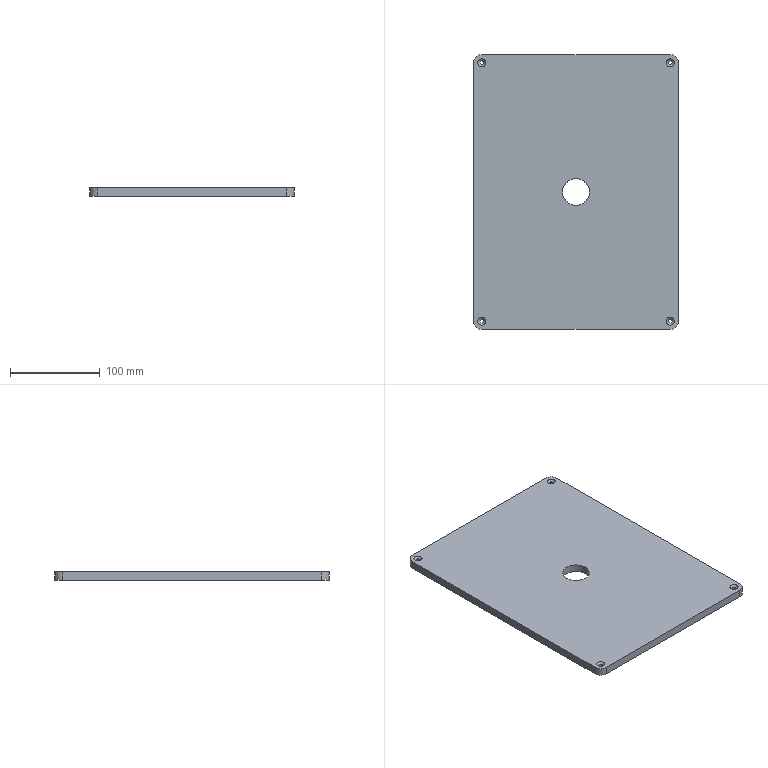Part | STEP file | Substructure | 1 solid | 19 faces | box 228 x 306 x 9 mm | volume 620161 mm3 | cylinder 9 | plane 6 | cone 4 | commonest cylinder face diameters 4.5 x4 18 x4 30 x1
STEP:
#1=CARTESIAN_POINT('',(0.,0.,0.));
#2=DIRECTION('',(0.,0.,1.));
#3=DIRECTION('',(1.,0.,0.));
#4=AXIS2_PLACEMENT_3D('',#1,#2,#3);
#5=CARTESIAN_POINT('',(-105.,-153.,0.));
#6=VERTEX_POINT('',#5);
#7=CARTESIAN_POINT('',(-105.,-153.,-9.));
#8=VERTEX_POINT('',#7);
#9=CARTESIAN_POINT('',(-105.,-153.,0.));
#10=DIRECTION('',(0.,0.,-1.));
#11=VECTOR('',#10,1.);
#12=LINE('',#9,#11);
#13=CARTESIAN_POINT('',(-105.,-153.,0.));
#14=DIRECTION('',(0.,-1.,0.));
#15=DIRECTION('',(1.,0.,0.));
#16=AXIS2_PLACEMENT_3D('',#13,#14,#15);
#17=PLANE('',#16);
#18=CARTESIAN_POINT('',(0.,0.));
#19=DIRECTION('',(0.,-1.));
#20=VECTOR('',#19,1.);
#21=LINE('',#18,#20);
#22=(GEOMETRIC_REPRESENTATION_CONTEXT(2)PARAMETRIC_REPRESENTATION_CONTEXT()REPRESENTATION_CONTEXT('',''));
#23=DEFINITIONAL_REPRESENTATION('',(#21),#22);
#24=PCURVE('',#17,#23);
#25=CARTESIAN_POINT('',(-105.,-144.,0.));
#26=DIRECTION('',(0.,0.,1.));
#27=DIRECTION('',(1.,0.,0.));
#28=AXIS2_PLACEMENT_3D('',#25,#26,#27);
#29=CYLINDRICAL_SURFACE('',#28,9.);
#30=CARTESIAN_POINT('',(4.712,0.));
#31=DIRECTION('',(0.,-1.));
#32=VECTOR('',#31,1.);
#33=LINE('',#30,#32);
#34=(GEOMETRIC_REPRESENTATION_CONTEXT(2)PARAMETRIC_REPRESENTATION_CONTEXT()REPRESENTATION_CONTEXT('',''));
#35=DEFINITIONAL_REPRESENTATION('',(#33),#34);
#36=PCURVE('',#29,#35);
#37=SURFACE_CURVE('',#12,(#24,#36),.PCURVE_S1.);
#38=EDGE_CURVE('',#6,#8,#37,.T.);
#39=ORIENTED_EDGE('',*,*,#38,.T.);
#40=CARTESIAN_POINT('',(105.,-153.,-9.));
#41=VERTEX_POINT('',#40);
#42=CARTESIAN_POINT('',(-105.,-153.,-9.));
#43=DIRECTION('',(1.,0.,0.));
#44=VECTOR('',#43,1.);
#45=LINE('',#42,#44);
#46=CARTESIAN_POINT('',(0.,-9.));
#47=DIRECTION('',(1.,0.));
#48=VECTOR('',#47,1.);
#49=LINE('',#46,#48);
#50=(GEOMETRIC_REPRESENTATION_CONTEXT(2)PARAMETRIC_REPRESENTATION_CONTEXT()REPRESENTATION_CONTEXT('',''));
#51=DEFINITIONAL_REPRESENTATION('',(#49),#50);
#52=PCURVE('',#17,#51);
#53=CARTESIAN_POINT('',(0.,0.,-9.));
#54=DIRECTION('',(0.,0.,1.));
#55=DIRECTION('',(1.,0.,0.));
#56=AXIS2_PLACEMENT_3D('',#53,#54,#55);
#57=PLANE('',#56);
#58=CARTESIAN_POINT('',(-105.,-153.));
#59=DIRECTION('',(1.,0.));
#60=VECTOR('',#59,1.);
#61=LINE('',#58,#60);
#62=(GEOMETRIC_REPRESENTATION_CONTEXT(2)PARAMETRIC_REPRESENTATION_CONTEXT()REPRESENTATION_CONTEXT('',''));
#63=DEFINITIONAL_REPRESENTATION('',(#61),#62);
#64=PCURVE('',#57,#63);
#65=SURFACE_CURVE('',#45,(#52,#64),.PCURVE_S1.);
#66=EDGE_CURVE('',#8,#41,#65,.T.);
#67=ORIENTED_EDGE('',*,*,#66,.T.);
#68=CARTESIAN_POINT('',(105.,-153.,0.));
#69=VERTEX_POINT('',#68);
#70=CARTESIAN_POINT('',(105.,-153.,0.));
#71=DIRECTION('',(0.,0.,-1.));
#72=VECTOR('',#71,1.);
#73=LINE('',#70,#72);
#74=CARTESIAN_POINT('',(210.,0.));
#75=DIRECTION('',(0.,-1.));
#76=VECTOR('',#75,1.);
#77=LINE('',#74,#76);
#78=(GEOMETRIC_REPRESENTATION_CONTEXT(2)PARAMETRIC_REPRESENTATION_CONTEXT()REPRESENTATION_CONTEXT('',''));
#79=DEFINITIONAL_REPRESENTATION('',(#77),#78);
#80=PCURVE('',#17,#79);
#81=CARTESIAN_POINT('',(105.,-144.,0.));
#82=DIRECTION('',(0.,0.,1.));
#83=DIRECTION('',(1.,0.,0.));
#84=AXIS2_PLACEMENT_3D('',#81,#82,#83);
#85=CYLINDRICAL_SURFACE('',#84,9.);
#86=CARTESIAN_POINT('',(4.712,0.));
#87=DIRECTION('',(0.,-1.));
#88=VECTOR('',#87,1.);
#89=LINE('',#86,#88);
#90=(GEOMETRIC_REPRESENTATION_CONTEXT(2)PARAMETRIC_REPRESENTATION_CONTEXT()REPRESENTATION_CONTEXT('',''));
#91=DEFINITIONAL_REPRESENTATION('',(#89),#90);
#92=PCURVE('',#85,#91);
#93=SURFACE_CURVE('',#73,(#80,#92),.PCURVE_S1.);
#94=EDGE_CURVE('',#69,#41,#93,.T.);
#95=ORIENTED_EDGE('',*,*,#94,.F.);
#96=CARTESIAN_POINT('',(-105.,-153.,0.));
#97=DIRECTION('',(1.,0.,0.));
#98=VECTOR('',#97,1.);
#99=LINE('',#96,#98);
#100=CARTESIAN_POINT('',(0.,0.));
#101=DIRECTION('',(1.,0.));
#102=VECTOR('',#101,1.);
#103=LINE('',#100,#102);
#104=(GEOMETRIC_REPRESENTATION_CONTEXT(2)PARAMETRIC_REPRESENTATION_CONTEXT()REPRESENTATION_CONTEXT('',''));
#105=DEFINITIONAL_REPRESENTATION('',(#103),#104);
#106=PCURVE('',#17,#105);
#107=CARTESIAN_POINT('',(0.,0.,0.));
#108=DIRECTION('',(0.,0.,1.));
#109=DIRECTION('',(1.,0.,0.));
#110=AXIS2_PLACEMENT_3D('',#107,#108,#109);
#111=PLANE('',#110);
#112=CARTESIAN_POINT('',(-105.,-153.));
#113=DIRECTION('',(1.,0.));
#114=VECTOR('',#113,1.);
#115=LINE('',#112,#114);
#116=(GEOMETRIC_REPRESENTATION_CONTEXT(2)PARAMETRIC_REPRESENTATION_CONTEXT()REPRESENTATION_CONTEXT('',''));
#117=DEFINITIONAL_REPRESENTATION('',(#115),#116);
#118=PCURVE('',#111,#117);
#119=SURFACE_CURVE('',#99,(#106,#118),.PCURVE_S1.);
#120=EDGE_CURVE('',#6,#69,#119,.T.);
#121=ORIENTED_EDGE('',*,*,#120,.F.);
#122=EDGE_LOOP('',(#39,#67,#95,#121));
#123=FACE_BOUND('',#122,.T.);
#124=ADVANCED_FACE('',(#123),#17,.T.);
#125=CARTESIAN_POINT('',(-114.,-144.,0.));
#126=VERTEX_POINT('',#125);
#127=CARTESIAN_POINT('',(-114.,-144.,-9.));
#128=VERTEX_POINT('',#127);
#129=CARTESIAN_POINT('',(-114.,-144.,0.));
#130=DIRECTION('',(0.,0.,-1.));
#131=VECTOR('',#130,1.);
#132=LINE('',#129,#131);
#133=CARTESIAN_POINT('',(3.142,0.));
#134=DIRECTION('',(0.,-1.));
#135=VECTOR('',#134,1.);
#136=LINE('',#133,#135);
#137=(GEOMETRIC_REPRESENTATION_CONTEXT(2)PARAMETRIC_REPRESENTATION_CONTEXT()REPRESENTATION_CONTEXT('',''));
#138=DEFINITIONAL_REPRESENTATION('',(#136),#137);
#139=PCURVE('',#29,#138);
#140=CARTESIAN_POINT('',(-114.,144.,0.));
#141=DIRECTION('',(-1.,0.,0.));
#142=DIRECTION('',(0.,-1.,0.));
#143=AXIS2_PLACEMENT_3D('',#140,#141,#142);
#144=PLANE('',#143);
#145=CARTESIAN_POINT('',(288.,0.));
#146=DIRECTION('',(0.,-1.));
#147=VECTOR('',#146,1.);
#148=LINE('',#145,#147);
#149=(GEOMETRIC_REPRESENTATION_CONTEXT(2)PARAMETRIC_REPRESENTATION_CONTEXT()REPRESENTATION_CONTEXT('',''));
#150=DEFINITIONAL_REPRESENTATION('',(#148),#149);
#151=PCURVE('',#144,#150);
#152=SURFACE_CURVE('',#132,(#139,#151),.PCURVE_S1.);
#153=EDGE_CURVE('',#126,#128,#152,.T.);
#154=ORIENTED_EDGE('',*,*,#153,.T.);
#155=CARTESIAN_POINT('',(-105.,-144.,-9.));
#156=DIRECTION('',(0.,0.,1.));
#157=DIRECTION('',(1.,0.,0.));
#158=AXIS2_PLACEMENT_3D('',#155,#156,#157);
#159=CIRCLE('',#158,9.);
#160=CARTESIAN_POINT('',(0.,-9.));
#161=DIRECTION('',(1.,0.));
#162=VECTOR('',#161,1.);
#163=LINE('',#160,#162);
#164=(GEOMETRIC_REPRESENTATION_CONTEXT(2)PARAMETRIC_REPRESENTATION_CONTEXT()REPRESENTATION_CONTEXT('',''));
#165=DEFINITIONAL_REPRESENTATION('',(#163),#164);
#166=PCURVE('',#29,#165);
#167=CARTESIAN_POINT('',(-105.,-144.));
#168=DIRECTION('',(1.,0.));
#169=AXIS2_PLACEMENT_2D('',#167,#168);
#170=CIRCLE('',#169,9.);
#171=(GEOMETRIC_REPRESENTATION_CONTEXT(2)PARAMETRIC_REPRESENTATION_CONTEXT()REPRESENTATION_CONTEXT('',''));
#172=DEFINITIONAL_REPRESENTATION('',(#170),#171);
#173=PCURVE('',#57,#172);
#174=SURFACE_CURVE('',#159,(#166,#173),.PCURVE_S1.);
#175=EDGE_CURVE('',#128,#8,#174,.T.);
#176=ORIENTED_EDGE('',*,*,#175,.T.);
#177=ORIENTED_EDGE('',*,*,#38,.F.);
#178=CARTESIAN_POINT('',(-105.,-144.,0.));
#179=DIRECTION('',(0.,0.,1.));
#180=DIRECTION('',(1.,0.,0.));
#181=AXIS2_PLACEMENT_3D('',#178,#179,#180);
#182=CIRCLE('',#181,9.);
#183=CARTESIAN_POINT('',(0.,0.));
#184=DIRECTION('',(1.,0.));
#185=VECTOR('',#184,1.);
#186=LINE('',#183,#185);
#187=(GEOMETRIC_REPRESENTATION_CONTEXT(2)PARAMETRIC_REPRESENTATION_CONTEXT()REPRESENTATION_CONTEXT('',''));
#188=DEFINITIONAL_REPRESENTATION('',(#186),#187);
#189=PCURVE('',#29,#188);
#190=CARTESIAN_POINT('',(-105.,-144.));
#191=DIRECTION('',(1.,0.));
#192=AXIS2_PLACEMENT_2D('',#190,#191);
#193=CIRCLE('',#192,9.);
#194=(GEOMETRIC_REPRESENTATION_CONTEXT(2)PARAMETRIC_REPRESENTATION_CONTEXT()REPRESENTATION_CONTEXT('',''));
#195=DEFINITIONAL_REPRESENTATION('',(#193),#194);
#196=PCURVE('',#111,#195);
#197=SURFACE_CURVE('',#182,(#189,#196),.PCURVE_S1.);
#198=EDGE_CURVE('',#126,#6,#197,.T.);
#199=ORIENTED_EDGE('',*,*,#198,.F.);
#200=EDGE_LOOP('',(#154,#176,#177,#199));
#201=FACE_BOUND('',#200,.T.);
#202=ADVANCED_FACE('',(#201),#29,.T.);
#203=ORIENTED_EDGE('',*,*,#94,.T.);
#204=CARTESIAN_POINT('',(114.,-144.,-9.));
#205=VERTEX_POINT('',#204);
#206=CARTESIAN_POINT('',(105.,-144.,-9.));
#207=DIRECTION('',(0.,0.,1.));
#208=DIRECTION('',(1.,0.,0.));
#209=AXIS2_PLACEMENT_3D('',#206,#207,#208);
#210=CIRCLE('',#209,9.);
#211=CARTESIAN_POINT('',(0.,-9.));
#212=DIRECTION('',(1.,0.));
#213=VECTOR('',#212,1.);
#214=LINE('',#211,#213);
#215=(GEOMETRIC_REPRESENTATION_CONTEXT(2)PARAMETRIC_REPRESENTATION_CONTEXT()REPRESENTATION_CONTEXT('',''));
#216=DEFINITIONAL_REPRESENTATION('',(#214),#215);
#217=PCURVE('',#85,#216);
#218=CARTESIAN_POINT('',(105.,-144.));
#219=DIRECTION('',(1.,0.));
#220=AXIS2_PLACEMENT_2D('',#218,#219);
#221=CIRCLE('',#220,9.);
#222=(GEOMETRIC_REPRESENTATION_CONTEXT(2)PARAMETRIC_REPRESENTATION_CONTEXT()REPRESENTATION_CONTEXT('',''));
#223=DEFINITIONAL_REPRESENTATION('',(#221),#222);
#224=PCURVE('',#57,#223);
#225=SURFACE_CURVE('',#210,(#217,#224),.PCURVE_S1.);
#226=EDGE_CURVE('',#41,#205,#225,.T.);
#227=ORIENTED_EDGE('',*,*,#226,.T.);
#228=CARTESIAN_POINT('',(114.,-144.,0.));
#229=VERTEX_POINT('',#228);
#230=CARTESIAN_POINT('',(114.,-144.,0.));
#231=DIRECTION('',(0.,0.,-1.));
#232=VECTOR('',#231,1.);
#233=LINE('',#230,#232);
#234=CARTESIAN_POINT('',(6.283,0.));
#235=DIRECTION('',(0.,-1.));
#236=VECTOR('',#235,1.);
#237=LINE('',#234,#236);
#238=(GEOMETRIC_REPRESENTATION_CONTEXT(2)PARAMETRIC_REPRESENTATION_CONTEXT()REPRESENTATION_CONTEXT('',''));
#239=DEFINITIONAL_REPRESENTATION('',(#237),#238);
#240=PCURVE('',#85,#239);
#241=CARTESIAN_POINT('',(114.,-144.,0.));
#242=DIRECTION('',(1.,0.,0.));
#243=DIRECTION('',(0.,1.,0.));
#244=AXIS2_PLACEMENT_3D('',#241,#242,#243);
#245=PLANE('',#244);
#246=CARTESIAN_POINT('',(0.,0.));
#247=DIRECTION('',(0.,-1.));
#248=VECTOR('',#247,1.);
#249=LINE('',#246,#248);
#250=(GEOMETRIC_REPRESENTATION_CONTEXT(2)PARAMETRIC_REPRESENTATION_CONTEXT()REPRESENTATION_CONTEXT('',''));
#251=DEFINITIONAL_REPRESENTATION('',(#249),#250);
#252=PCURVE('',#245,#251);
#253=SURFACE_CURVE('',#233,(#240,#252),.PCURVE_S1.);
#254=EDGE_CURVE('',#229,#205,#253,.T.);
#255=ORIENTED_EDGE('',*,*,#254,.F.);
#256=CARTESIAN_POINT('',(105.,-144.,0.));
#257=DIRECTION('',(0.,0.,1.));
#258=DIRECTION('',(1.,0.,0.));
#259=AXIS2_PLACEMENT_3D('',#256,#257,#258);
#260=CIRCLE('',#259,9.);
#261=CARTESIAN_POINT('',(0.,0.));
#262=DIRECTION('',(1.,0.));
#263=VECTOR('',#262,1.);
#264=LINE('',#261,#263);
#265=(GEOMETRIC_REPRESENTATION_CONTEXT(2)PARAMETRIC_REPRESENTATION_CONTEXT()REPRESENTATION_CONTEXT('',''));
#266=DEFINITIONAL_REPRESENTATION('',(#264),#265);
#267=PCURVE('',#85,#266);
#268=CARTESIAN_POINT('',(105.,-144.));
#269=DIRECTION('',(1.,0.));
#270=AXIS2_PLACEMENT_2D('',#268,#269);
#271=CIRCLE('',#270,9.);
#272=(GEOMETRIC_REPRESENTATION_CONTEXT(2)PARAMETRIC_REPRESENTATION_CONTEXT()REPRESENTATION_CONTEXT('',''));
#273=DEFINITIONAL_REPRESENTATION('',(#271),#272);
#274=PCURVE('',#111,#273);
#275=SURFACE_CURVE('',#260,(#267,#274),.PCURVE_S1.);
#276=EDGE_CURVE('',#69,#229,#275,.T.);
#277=ORIENTED_EDGE('',*,*,#276,.F.);
#278=EDGE_LOOP('',(#203,#227,#255,#277));
#279=FACE_BOUND('',#278,.T.);
#280=ADVANCED_FACE('',(#279),#85,.T.);
#281=ORIENTED_EDGE('',*,*,#120,.T.);
#282=ORIENTED_EDGE('',*,*,#276,.T.);
#283=CARTESIAN_POINT('',(114.,144.,0.));
#284=VERTEX_POINT('',#283);
#285=CARTESIAN_POINT('',(114.,-144.,0.));
#286=DIRECTION('',(0.,1.,0.));
#287=VECTOR('',#286,1.);
#288=LINE('',#285,#287);
#289=CARTESIAN_POINT('',(114.,-144.));
#290=DIRECTION('',(0.,1.));
#291=VECTOR('',#290,1.);
#292=LINE('',#289,#291);
#293=(GEOMETRIC_REPRESENTATION_CONTEXT(2)PARAMETRIC_REPRESENTATION_CONTEXT()REPRESENTATION_CONTEXT('',''));
#294=DEFINITIONAL_REPRESENTATION('',(#292),#293);
#295=PCURVE('',#111,#294);
#296=CARTESIAN_POINT('',(0.,0.));
#297=DIRECTION('',(1.,0.));
#298=VECTOR('',#297,1.);
#299=LINE('',#296,#298);
#300=(GEOMETRIC_REPRESENTATION_CONTEXT(2)PARAMETRIC_REPRESENTATION_CONTEXT()REPRESENTATION_CONTEXT('',''));
#301=DEFINITIONAL_REPRESENTATION('',(#299),#300);
#302=PCURVE('',#245,#301);
#303=SURFACE_CURVE('',#288,(#295,#302),.PCURVE_S1.);
#304=EDGE_CURVE('',#229,#284,#303,.T.);
#305=ORIENTED_EDGE('',*,*,#304,.T.);
#306=CARTESIAN_POINT('',(105.,153.,0.));
#307=VERTEX_POINT('',#306);
#308=CARTESIAN_POINT('',(105.,144.,0.));
#309=DIRECTION('',(0.,0.,1.));
#310=DIRECTION('',(1.,0.,0.));
#311=AXIS2_PLACEMENT_3D('',#308,#309,#310);
#312=CIRCLE('',#311,9.);
#313=CARTESIAN_POINT('',(105.,144.));
#314=DIRECTION('',(1.,0.));
#315=AXIS2_PLACEMENT_2D('',#313,#314);
#316=CIRCLE('',#315,9.);
#317=(GEOMETRIC_REPRESENTATION_CONTEXT(2)PARAMETRIC_REPRESENTATION_CONTEXT()REPRESENTATION_CONTEXT('',''));
#318=DEFINITIONAL_REPRESENTATION('',(#316),#317);
#319=PCURVE('',#111,#318);
#320=CARTESIAN_POINT('',(105.,144.,0.));
#321=DIRECTION('',(0.,0.,1.));
#322=DIRECTION('',(1.,0.,0.));
#323=AXIS2_PLACEMENT_3D('',#320,#321,#322);
#324=CYLINDRICAL_SURFACE('',#323,9.);
#325=CARTESIAN_POINT('',(0.,0.));
#326=DIRECTION('',(1.,0.));
#327=VECTOR('',#326,1.);
#328=LINE('',#325,#327);
#329=(GEOMETRIC_REPRESENTATION_CONTEXT(2)PARAMETRIC_REPRESENTATION_CONTEXT()REPRESENTATION_CONTEXT('',''));
#330=DEFINITIONAL_REPRESENTATION('',(#328),#329);
#331=PCURVE('',#324,#330);
#332=SURFACE_CURVE('',#312,(#319,#331),.PCURVE_S1.);
#333=EDGE_CURVE('',#284,#307,#332,.T.);
#334=ORIENTED_EDGE('',*,*,#333,.T.);
#335=CARTESIAN_POINT('',(-105.,153.,0.));
#336=VERTEX_POINT('',#335);
#337=CARTESIAN_POINT('',(105.,153.,0.));
#338=DIRECTION('',(-1.,0.,0.));
#339=VECTOR('',#338,1.);
#340=LINE('',#337,#339);
#341=CARTESIAN_POINT('',(105.,153.));
#342=DIRECTION('',(-1.,0.));
#343=VECTOR('',#342,1.);
#344=LINE('',#341,#343);
#345=(GEOMETRIC_REPRESENTATION_CONTEXT(2)PARAMETRIC_REPRESENTATION_CONTEXT()REPRESENTATION_CONTEXT('',''));
#346=DEFINITIONAL_REPRESENTATION('',(#344),#345);
#347=PCURVE('',#111,#346);
#348=CARTESIAN_POINT('',(105.,153.,0.));
#349=DIRECTION('',(0.,1.,0.));
#350=DIRECTION('',(-1.,0.,0.));
#351=AXIS2_PLACEMENT_3D('',#348,#349,#350);
#352=PLANE('',#351);
#353=CARTESIAN_POINT('',(0.,0.));
#354=DIRECTION('',(1.,0.));
#355=VECTOR('',#354,1.);
#356=LINE('',#353,#355);
#357=(GEOMETRIC_REPRESENTATION_CONTEXT(2)PARAMETRIC_REPRESENTATION_CONTEXT()REPRESENTATION_CONTEXT('',''));
#358=DEFINITIONAL_REPRESENTATION('',(#356),#357);
#359=PCURVE('',#352,#358);
#360=SURFACE_CURVE('',#340,(#347,#359),.PCURVE_S1.);
#361=EDGE_CURVE('',#307,#336,#360,.T.);
#362=ORIENTED_EDGE('',*,*,#361,.T.);
#363=CARTESIAN_POINT('',(-114.,144.,0.));
#364=VERTEX_POINT('',#363);
#365=CARTESIAN_POINT('',(-105.,144.,0.));
#366=DIRECTION('',(0.,0.,1.));
#367=DIRECTION('',(1.,0.,0.));
#368=AXIS2_PLACEMENT_3D('',#365,#366,#367);
#369=CIRCLE('',#368,9.);
#370=CARTESIAN_POINT('',(-105.,144.));
#371=DIRECTION('',(1.,0.));
#372=AXIS2_PLACEMENT_2D('',#370,#371);
#373=CIRCLE('',#372,9.);
#374=(GEOMETRIC_REPRESENTATION_CONTEXT(2)PARAMETRIC_REPRESENTATION_CONTEXT()REPRESENTATION_CONTEXT('',''));
#375=DEFINITIONAL_REPRESENTATION('',(#373),#374);
#376=PCURVE('',#111,#375);
#377=CARTESIAN_POINT('',(-105.,144.,0.));
#378=DIRECTION('',(0.,0.,1.));
#379=DIRECTION('',(1.,0.,0.));
#380=AXIS2_PLACEMENT_3D('',#377,#378,#379);
#381=CYLINDRICAL_SURFACE('',#380,9.);
#382=CARTESIAN_POINT('',(0.,0.));
#383=DIRECTION('',(1.,0.));
#384=VECTOR('',#383,1.);
#385=LINE('',#382,#384);
#386=(GEOMETRIC_REPRESENTATION_CONTEXT(2)PARAMETRIC_REPRESENTATION_CONTEXT()REPRESENTATION_CONTEXT('',''));
#387=DEFINITIONAL_REPRESENTATION('',(#385),#386);
#388=PCURVE('',#381,#387);
#389=SURFACE_CURVE('',#369,(#376,#388),.PCURVE_S1.);
#390=EDGE_CURVE('',#336,#364,#389,.T.);
#391=ORIENTED_EDGE('',*,*,#390,.T.);
#392=CARTESIAN_POINT('',(-114.,144.,0.));
#393=DIRECTION('',(0.,-1.,0.));
#394=VECTOR('',#393,1.);
#395=LINE('',#392,#394);
#396=CARTESIAN_POINT('',(-114.,144.));
#397=DIRECTION('',(0.,-1.));
#398=VECTOR('',#397,1.);
#399=LINE('',#396,#398);
#400=(GEOMETRIC_REPRESENTATION_CONTEXT(2)PARAMETRIC_REPRESENTATION_CONTEXT()REPRESENTATION_CONTEXT('',''));
#401=DEFINITIONAL_REPRESENTATION('',(#399),#400);
#402=PCURVE('',#111,#401);
#403=CARTESIAN_POINT('',(0.,0.));
#404=DIRECTION('',(1.,0.));
#405=VECTOR('',#404,1.);
#406=LINE('',#403,#405);
#407=(GEOMETRIC_REPRESENTATION_CONTEXT(2)PARAMETRIC_REPRESENTATION_CONTEXT()REPRESENTATION_CONTEXT('',''));
#408=DEFINITIONAL_REPRESENTATION('',(#406),#407);
#409=PCURVE('',#144,#408);
#410=SURFACE_CURVE('',#395,(#402,#409),.PCURVE_S1.);
#411=EDGE_CURVE('',#364,#126,#410,.T.);
#412=ORIENTED_EDGE('',*,*,#411,.T.);
#413=ORIENTED_EDGE('',*,*,#198,.T.);
#414=EDGE_LOOP('',(#281,#282,#305,#334,#362,#391,#412,#413));
#415=FACE_BOUND('',#414,.T.);
#416=CARTESIAN_POINT('',(-100.5,-144.,0.));
#417=VERTEX_POINT('',#416);
#418=CARTESIAN_POINT('',(-105.,-144.,0.));
#419=DIRECTION('',(0.,0.,1.));
#420=DIRECTION('',(1.,0.,0.));
#421=AXIS2_PLACEMENT_3D('',#418,#419,#420);
#422=CIRCLE('',#421,4.5);
#423=CARTESIAN_POINT('',(-105.,-144.));
#424=DIRECTION('',(1.,0.));
#425=AXIS2_PLACEMENT_2D('',#423,#424);
#426=CIRCLE('',#425,4.5);
#427=(GEOMETRIC_REPRESENTATION_CONTEXT(2)PARAMETRIC_REPRESENTATION_CONTEXT()REPRESENTATION_CONTEXT('',''));
#428=DEFINITIONAL_REPRESENTATION('',(#426),#427);
#429=PCURVE('',#111,#428);
#430=CARTESIAN_POINT('',(-105.,-144.,0.));
#431=DIRECTION('',(0.,0.,1.));
#432=DIRECTION('',(1.,0.,0.));
#433=AXIS2_PLACEMENT_3D('',#430,#431,#432);
#434=CONICAL_SURFACE('',#433,4.5,0.7854);
#435=CARTESIAN_POINT('',(0.,0.));
#436=DIRECTION('',(1.,0.));
#437=VECTOR('',#436,1.);
#438=LINE('',#435,#437);
#439=(GEOMETRIC_REPRESENTATION_CONTEXT(2)PARAMETRIC_REPRESENTATION_CONTEXT()REPRESENTATION_CONTEXT('',''));
#440=DEFINITIONAL_REPRESENTATION('',(#438),#439);
#441=PCURVE('',#434,#440);
#442=SURFACE_CURVE('',#422,(#429,#441),.PCURVE_S1.);
#443=EDGE_CURVE('',#417,#417,#442,.T.);
#444=ORIENTED_EDGE('',*,*,#443,.F.);
#445=EDGE_LOOP('',(#444));
#446=FACE_BOUND('',#445,.T.);
#447=CARTESIAN_POINT('',(109.5,-144.,0.));
#448=VERTEX_POINT('',#447);
#449=CARTESIAN_POINT('',(105.,-144.,0.));
#450=DIRECTION('',(0.,0.,1.));
#451=DIRECTION('',(1.,0.,0.));
#452=AXIS2_PLACEMENT_3D('',#449,#450,#451);
#453=CIRCLE('',#452,4.5);
#454=CARTESIAN_POINT('',(105.,-144.));
#455=DIRECTION('',(1.,0.));
#456=AXIS2_PLACEMENT_2D('',#454,#455);
#457=CIRCLE('',#456,4.5);
#458=(GEOMETRIC_REPRESENTATION_CONTEXT(2)PARAMETRIC_REPRESENTATION_CONTEXT()REPRESENTATION_CONTEXT('',''));
#459=DEFINITIONAL_REPRESENTATION('',(#457),#458);
#460=PCURVE('',#111,#459);
#461=CARTESIAN_POINT('',(105.,-144.,0.));
#462=DIRECTION('',(0.,0.,1.));
#463=DIRECTION('',(1.,0.,0.));
#464=AXIS2_PLACEMENT_3D('',#461,#462,#463);
#465=CONICAL_SURFACE('',#464,4.5,0.7854);
#466=CARTESIAN_POINT('',(0.,0.));
#467=DIRECTION('',(1.,0.));
#468=VECTOR('',#467,1.);
#469=LINE('',#466,#468);
#470=(GEOMETRIC_REPRESENTATION_CONTEXT(2)PARAMETRIC_REPRESENTATION_CONTEXT()REPRESENTATION_CONTEXT('',''));
#471=DEFINITIONAL_REPRESENTATION('',(#469),#470);
#472=PCURVE('',#465,#471);
#473=SURFACE_CURVE('',#453,(#460,#472),.PCURVE_S1.);
#474=EDGE_CURVE('',#448,#448,#473,.T.);
#475=ORIENTED_EDGE('',*,*,#474,.F.);
#476=EDGE_LOOP('',(#475));
#477=FACE_BOUND('',#476,.T.);
#478=CARTESIAN_POINT('',(-100.5,144.,0.));
#479=VERTEX_POINT('',#478);
#480=CARTESIAN_POINT('',(-105.,144.,0.));
#481=DIRECTION('',(0.,0.,1.));
#482=DIRECTION('',(1.,0.,0.));
#483=AXIS2_PLACEMENT_3D('',#480,#481,#482);
#484=CIRCLE('',#483,4.5);
#485=CARTESIAN_POINT('',(-105.,144.));
#486=DIRECTION('',(1.,0.));
#487=AXIS2_PLACEMENT_2D('',#485,#486);
#488=CIRCLE('',#487,4.5);
#489=(GEOMETRIC_REPRESENTATION_CONTEXT(2)PARAMETRIC_REPRESENTATION_CONTEXT()REPRESENTATION_CONTEXT('',''));
#490=DEFINITIONAL_REPRESENTATION('',(#488),#489);
#491=PCURVE('',#111,#490);
#492=CARTESIAN_POINT('',(-105.,144.,0.));
#493=DIRECTION('',(0.,0.,1.));
#494=DIRECTION('',(1.,0.,0.));
#495=AXIS2_PLACEMENT_3D('',#492,#493,#494);
#496=CONICAL_SURFACE('',#495,4.5,0.7854);
#497=CARTESIAN_POINT('',(0.,0.));
#498=DIRECTION('',(1.,0.));
#499=VECTOR('',#498,1.);
#500=LINE('',#497,#499);
#501=(GEOMETRIC_REPRESENTATION_CONTEXT(2)PARAMETRIC_REPRESENTATION_CONTEXT()REPRESENTATION_CONTEXT('',''));
#502=DEFINITIONAL_REPRESENTATION('',(#500),#501);
#503=PCURVE('',#496,#502);
#504=SURFACE_CURVE('',#484,(#491,#503),.PCURVE_S1.);
#505=EDGE_CURVE('',#479,#479,#504,.T.);
#506=ORIENTED_EDGE('',*,*,#505,.F.);
#507=EDGE_LOOP('',(#506));
#508=FACE_BOUND('',#507,.T.);
#509=CARTESIAN_POINT('',(15.,0.,0.));
#510=VERTEX_POINT('',#509);
#511=CARTESIAN_POINT('',(0.,0.,0.));
#512=DIRECTION('',(0.,0.,1.));
#513=DIRECTION('',(1.,0.,0.));
#514=AXIS2_PLACEMENT_3D('',#511,#512,#513);
#515=CIRCLE('',#514,15.);
#516=CARTESIAN_POINT('',(0.,0.));
#517=DIRECTION('',(1.,0.));
#518=AXIS2_PLACEMENT_2D('',#516,#517);
#519=CIRCLE('',#518,15.);
#520=(GEOMETRIC_REPRESENTATION_CONTEXT(2)PARAMETRIC_REPRESENTATION_CONTEXT()REPRESENTATION_CONTEXT('',''));
#521=DEFINITIONAL_REPRESENTATION('',(#519),#520);
#522=PCURVE('',#111,#521);
#523=CARTESIAN_POINT('',(0.,0.,0.));
#524=DIRECTION('',(0.,0.,1.));
#525=DIRECTION('',(1.,0.,0.));
#526=AXIS2_PLACEMENT_3D('',#523,#524,#525);
#527=CYLINDRICAL_SURFACE('',#526,15.);
#528=CARTESIAN_POINT('',(0.,0.));
#529=DIRECTION('',(1.,0.));
#530=VECTOR('',#529,1.);
#531=LINE('',#528,#530);
#532=(GEOMETRIC_REPRESENTATION_CONTEXT(2)PARAMETRIC_REPRESENTATION_CONTEXT()REPRESENTATION_CONTEXT('',''));
#533=DEFINITIONAL_REPRESENTATION('',(#531),#532);
#534=PCURVE('',#527,#533);
#535=SURFACE_CURVE('',#515,(#522,#534),.PCURVE_S1.);
#536=EDGE_CURVE('',#510,#510,#535,.T.);
#537=ORIENTED_EDGE('',*,*,#536,.F.);
#538=EDGE_LOOP('',(#537));
#539=FACE_BOUND('',#538,.T.);
#540=CARTESIAN_POINT('',(109.5,144.,0.));
#541=VERTEX_POINT('',#540);
#542=CARTESIAN_POINT('',(105.,144.,0.));
#543=DIRECTION('',(0.,0.,1.));
#544=DIRECTION('',(1.,0.,0.));
#545=AXIS2_PLACEMENT_3D('',#542,#543,#544);
#546=CIRCLE('',#545,4.5);
#547=CARTESIAN_POINT('',(105.,144.));
#548=DIRECTION('',(1.,0.));
#549=AXIS2_PLACEMENT_2D('',#547,#548);
#550=CIRCLE('',#549,4.5);
#551=(GEOMETRIC_REPRESENTATION_CONTEXT(2)PARAMETRIC_REPRESENTATION_CONTEXT()REPRESENTATION_CONTEXT('',''));
#552=DEFINITIONAL_REPRESENTATION('',(#550),#551);
#553=PCURVE('',#111,#552);
#554=CARTESIAN_POINT('',(105.,144.,0.));
#555=DIRECTION('',(0.,0.,1.));
#556=DIRECTION('',(1.,0.,0.));
#557=AXIS2_PLACEMENT_3D('',#554,#555,#556);
#558=CONICAL_SURFACE('',#557,4.5,0.7854);
#559=CARTESIAN_POINT('',(0.,0.));
#560=DIRECTION('',(1.,0.));
#561=VECTOR('',#560,1.);
#562=LINE('',#559,#561);
#563=(GEOMETRIC_REPRESENTATION_CONTEXT(2)PARAMETRIC_REPRESENTATION_CONTEXT()REPRESENTATION_CONTEXT('',''));
#564=DEFINITIONAL_REPRESENTATION('',(#562),#563);
#565=PCURVE('',#558,#564);
#566=SURFACE_CURVE('',#546,(#553,#565),.PCURVE_S1.);
#567=EDGE_CURVE('',#541,#541,#566,.T.);
#568=ORIENTED_EDGE('',*,*,#567,.F.);
#569=EDGE_LOOP('',(#568));
#570=FACE_BOUND('',#569,.T.);
#571=ADVANCED_FACE('',(#415,#446,#477,#508,#539,#570),#111,.T.);
#572=ORIENTED_EDGE('',*,*,#66,.T.);
#573=ORIENTED_EDGE('',*,*,#226,.T.);
#574=CARTESIAN_POINT('',(114.,144.,-9.));
#575=VERTEX_POINT('',#574);
#576=CARTESIAN_POINT('',(114.,-144.,-9.));
#577=DIRECTION('',(0.,1.,0.));
#578=VECTOR('',#577,1.);
#579=LINE('',#576,#578);
#580=CARTESIAN_POINT('',(114.,-144.));
#581=DIRECTION('',(0.,1.));
#582=VECTOR('',#581,1.);
#583=LINE('',#580,#582);
#584=(GEOMETRIC_REPRESENTATION_CONTEXT(2)PARAMETRIC_REPRESENTATION_CONTEXT()REPRESENTATION_CONTEXT('',''));
#585=DEFINITIONAL_REPRESENTATION('',(#583),#584);
#586=PCURVE('',#57,#585);
#587=CARTESIAN_POINT('',(0.,-9.));
#588=DIRECTION('',(1.,0.));
#589=VECTOR('',#588,1.);
#590=LINE('',#587,#589);
#591=(GEOMETRIC_REPRESENTATION_CONTEXT(2)PARAMETRIC_REPRESENTATION_CONTEXT()REPRESENTATION_CONTEXT('',''));
#592=DEFINITIONAL_REPRESENTATION('',(#590),#591);
#593=PCURVE('',#245,#592);
#594=SURFACE_CURVE('',#579,(#586,#593),.PCURVE_S1.);
#595=EDGE_CURVE('',#205,#575,#594,.T.);
#596=ORIENTED_EDGE('',*,*,#595,.T.);
#597=CARTESIAN_POINT('',(105.,153.,-9.));
#598=VERTEX_POINT('',#597);
#599=CARTESIAN_POINT('',(105.,144.,-9.));
#600=DIRECTION('',(0.,0.,1.));
#601=DIRECTION('',(1.,0.,0.));
#602=AXIS2_PLACEMENT_3D('',#599,#600,#601);
#603=CIRCLE('',#602,9.);
#604=CARTESIAN_POINT('',(105.,144.));
#605=DIRECTION('',(1.,0.));
#606=AXIS2_PLACEMENT_2D('',#604,#605);
#607=CIRCLE('',#606,9.);
#608=(GEOMETRIC_REPRESENTATION_CONTEXT(2)PARAMETRIC_REPRESENTATION_CONTEXT()REPRESENTATION_CONTEXT('',''));
#609=DEFINITIONAL_REPRESENTATION('',(#607),#608);
#610=PCURVE('',#57,#609);
#611=CARTESIAN_POINT('',(0.,-9.));
#612=DIRECTION('',(1.,0.));
#613=VECTOR('',#612,1.);
#614=LINE('',#611,#613);
#615=(GEOMETRIC_REPRESENTATION_CONTEXT(2)PARAMETRIC_REPRESENTATION_CONTEXT()REPRESENTATION_CONTEXT('',''));
#616=DEFINITIONAL_REPRESENTATION('',(#614),#615);
#617=PCURVE('',#324,#616);
#618=SURFACE_CURVE('',#603,(#610,#617),.PCURVE_S1.);
#619=EDGE_CURVE('',#575,#598,#618,.T.);
#620=ORIENTED_EDGE('',*,*,#619,.T.);
#621=CARTESIAN_POINT('',(-105.,153.,-9.));
#622=VERTEX_POINT('',#621);
#623=CARTESIAN_POINT('',(105.,153.,-9.));
#624=DIRECTION('',(-1.,0.,0.));
#625=VECTOR('',#624,1.);
#626=LINE('',#623,#625);
#627=CARTESIAN_POINT('',(105.,153.));
#628=DIRECTION('',(-1.,0.));
#629=VECTOR('',#628,1.);
#630=LINE('',#627,#629);
#631=(GEOMETRIC_REPRESENTATION_CONTEXT(2)PARAMETRIC_REPRESENTATION_CONTEXT()REPRESENTATION_CONTEXT('',''));
#632=DEFINITIONAL_REPRESENTATION('',(#630),#631);
#633=PCURVE('',#57,#632);
#634=CARTESIAN_POINT('',(0.,-9.));
#635=DIRECTION('',(1.,0.));
#636=VECTOR('',#635,1.);
#637=LINE('',#634,#636);
#638=(GEOMETRIC_REPRESENTATION_CONTEXT(2)PARAMETRIC_REPRESENTATION_CONTEXT()REPRESENTATION_CONTEXT('',''));
#639=DEFINITIONAL_REPRESENTATION('',(#637),#638);
#640=PCURVE('',#352,#639);
#641=SURFACE_CURVE('',#626,(#633,#640),.PCURVE_S1.);
#642=EDGE_CURVE('',#598,#622,#641,.T.);
#643=ORIENTED_EDGE('',*,*,#642,.T.);
#644=CARTESIAN_POINT('',(-114.,144.,-9.));
#645=VERTEX_POINT('',#644);
#646=CARTESIAN_POINT('',(-105.,144.,-9.));
#647=DIRECTION('',(0.,0.,1.));
#648=DIRECTION('',(1.,0.,0.));
#649=AXIS2_PLACEMENT_3D('',#646,#647,#648);
#650=CIRCLE('',#649,9.);
#651=CARTESIAN_POINT('',(-105.,144.));
#652=DIRECTION('',(1.,0.));
#653=AXIS2_PLACEMENT_2D('',#651,#652);
#654=CIRCLE('',#653,9.);
#655=(GEOMETRIC_REPRESENTATION_CONTEXT(2)PARAMETRIC_REPRESENTATION_CONTEXT()REPRESENTATION_CONTEXT('',''));
#656=DEFINITIONAL_REPRESENTATION('',(#654),#655);
#657=PCURVE('',#57,#656);
#658=CARTESIAN_POINT('',(0.,-9.));
#659=DIRECTION('',(1.,0.));
#660=VECTOR('',#659,1.);
#661=LINE('',#658,#660);
#662=(GEOMETRIC_REPRESENTATION_CONTEXT(2)PARAMETRIC_REPRESENTATION_CONTEXT()REPRESENTATION_CONTEXT('',''));
#663=DEFINITIONAL_REPRESENTATION('',(#661),#662);
#664=PCURVE('',#381,#663);
#665=SURFACE_CURVE('',#650,(#657,#664),.PCURVE_S1.);
#666=EDGE_CURVE('',#622,#645,#665,.T.);
#667=ORIENTED_EDGE('',*,*,#666,.T.);
#668=CARTESIAN_POINT('',(-114.,144.,-9.));
#669=DIRECTION('',(0.,-1.,0.));
#670=VECTOR('',#669,1.);
#671=LINE('',#668,#670);
#672=CARTESIAN_POINT('',(-114.,144.));
#673=DIRECTION('',(0.,-1.));
#674=VECTOR('',#673,1.);
#675=LINE('',#672,#674);
#676=(GEOMETRIC_REPRESENTATION_CONTEXT(2)PARAMETRIC_REPRESENTATION_CONTEXT()REPRESENTATION_CONTEXT('',''));
#677=DEFINITIONAL_REPRESENTATION('',(#675),#676);
#678=PCURVE('',#57,#677);
#679=CARTESIAN_POINT('',(0.,-9.));
#680=DIRECTION('',(1.,0.));
#681=VECTOR('',#680,1.);
#682=LINE('',#679,#681);
#683=(GEOMETRIC_REPRESENTATION_CONTEXT(2)PARAMETRIC_REPRESENTATION_CONTEXT()REPRESENTATION_CONTEXT('',''));
#684=DEFINITIONAL_REPRESENTATION('',(#682),#683);
#685=PCURVE('',#144,#684);
#686=SURFACE_CURVE('',#671,(#678,#685),.PCURVE_S1.);
#687=EDGE_CURVE('',#645,#128,#686,.T.);
#688=ORIENTED_EDGE('',*,*,#687,.T.);
#689=ORIENTED_EDGE('',*,*,#175,.T.);
#690=EDGE_LOOP('',(#572,#573,#596,#620,#643,#667,#688,#689));
#691=FACE_BOUND('',#690,.F.);
#692=CARTESIAN_POINT('',(-102.75,-144.,-9.));
#693=VERTEX_POINT('',#692);
#694=CARTESIAN_POINT('',(-105.,-144.,-9.));
#695=DIRECTION('',(0.,0.,-1.));
#696=DIRECTION('',(1.,0.,0.));
#697=AXIS2_PLACEMENT_3D('',#694,#695,#696);
#698=CIRCLE('',#697,2.25);
#699=CARTESIAN_POINT('',(-102.75,-144.));
#700=CARTESIAN_POINT('',(-102.75,-147.897));
#701=CARTESIAN_POINT('',(-106.125,-145.949));
#702=CARTESIAN_POINT('',(-109.5,-144.));
#703=CARTESIAN_POINT('',(-106.125,-142.051));
#704=CARTESIAN_POINT('',(-102.75,-140.103));
#705=CARTESIAN_POINT('',(-102.75,-144.));
#706=(BOUNDED_CURVE()B_SPLINE_CURVE(2,(#699,#700,#701,#702,#703,#704,#705),.UNSPECIFIED.,.T.,.F.)B_SPLINE_CURVE_WITH_KNOTS((1,2,2,2,2,1),(-2.094,0.,2.094,4.189,6.283,8.378),.UNSPECIFIED.)CURVE()GEOMETRIC_REPRESENTATION_ITEM()RATIONAL_B_SPLINE_CURVE((1.,0.5,1.,0.5,1.,0.5,1.))REPRESENTATION_ITEM(''));
#707=(GEOMETRIC_REPRESENTATION_CONTEXT(2)PARAMETRIC_REPRESENTATION_CONTEXT()REPRESENTATION_CONTEXT('',''));
#708=DEFINITIONAL_REPRESENTATION('',(#706),#707);
#709=PCURVE('',#57,#708);
#710=CARTESIAN_POINT('',(-105.,-144.,-2.25));
#711=DIRECTION('',(0.,0.,-1.));
#712=DIRECTION('',(1.,0.,0.));
#713=AXIS2_PLACEMENT_3D('',#710,#711,#712);
#714=CYLINDRICAL_SURFACE('',#713,2.25);
#715=CARTESIAN_POINT('',(0.,6.75));
#716=DIRECTION('',(1.,0.));
#717=VECTOR('',#716,1.);
#718=LINE('',#715,#717);
#719=(GEOMETRIC_REPRESENTATION_CONTEXT(2)PARAMETRIC_REPRESENTATION_CONTEXT()REPRESENTATION_CONTEXT('',''));
#720=DEFINITIONAL_REPRESENTATION('',(#718),#719);
#721=PCURVE('',#714,#720);
#722=SURFACE_CURVE('',#698,(#709,#721),.PCURVE_S1.);
#723=EDGE_CURVE('',#693,#693,#722,.T.);
#724=ORIENTED_EDGE('',*,*,#723,.T.);
#725=EDGE_LOOP('',(#724));
#726=FACE_BOUND('',#725,.F.);
#727=CARTESIAN_POINT('',(107.25,-144.,-9.));
#728=VERTEX_POINT('',#727);
#729=CARTESIAN_POINT('',(105.,-144.,-9.));
#730=DIRECTION('',(0.,0.,-1.));
#731=DIRECTION('',(1.,0.,0.));
#732=AXIS2_PLACEMENT_3D('',#729,#730,#731);
#733=CIRCLE('',#732,2.25);
#734=CARTESIAN_POINT('',(107.25,-144.));
#735=CARTESIAN_POINT('',(107.25,-147.897));
#736=CARTESIAN_POINT('',(103.875,-145.949));
#737=CARTESIAN_POINT('',(100.5,-144.));
#738=CARTESIAN_POINT('',(103.875,-142.051));
#739=CARTESIAN_POINT('',(107.25,-140.103));
#740=CARTESIAN_POINT('',(107.25,-144.));
#741=(BOUNDED_CURVE()B_SPLINE_CURVE(2,(#734,#735,#736,#737,#738,#739,#740),.UNSPECIFIED.,.T.,.F.)B_SPLINE_CURVE_WITH_KNOTS((1,2,2,2,2,1),(-2.094,0.,2.094,4.189,6.283,8.378),.UNSPECIFIED.)CURVE()GEOMETRIC_REPRESENTATION_ITEM()RATIONAL_B_SPLINE_CURVE((1.,0.5,1.,0.5,1.,0.5,1.))REPRESENTATION_ITEM(''));
#742=(GEOMETRIC_REPRESENTATION_CONTEXT(2)PARAMETRIC_REPRESENTATION_CONTEXT()REPRESENTATION_CONTEXT('',''));
#743=DEFINITIONAL_REPRESENTATION('',(#741),#742);
#744=PCURVE('',#57,#743);
#745=CARTESIAN_POINT('',(105.,-144.,-2.25));
#746=DIRECTION('',(0.,0.,-1.));
#747=DIRECTION('',(1.,0.,0.));
#748=AXIS2_PLACEMENT_3D('',#745,#746,#747);
#749=CYLINDRICAL_SURFACE('',#748,2.25);
#750=CARTESIAN_POINT('',(0.,6.75));
#751=DIRECTION('',(1.,0.));
#752=VECTOR('',#751,1.);
#753=LINE('',#750,#752);
#754=(GEOMETRIC_REPRESENTATION_CONTEXT(2)PARAMETRIC_REPRESENTATION_CONTEXT()REPRESENTATION_CONTEXT('',''));
#755=DEFINITIONAL_REPRESENTATION('',(#753),#754);
#756=PCURVE('',#749,#755);
#757=SURFACE_CURVE('',#733,(#744,#756),.PCURVE_S1.);
#758=EDGE_CURVE('',#728,#728,#757,.T.);
#759=ORIENTED_EDGE('',*,*,#758,.T.);
#760=EDGE_LOOP('',(#759));
#761=FACE_BOUND('',#760,.F.);
#762=CARTESIAN_POINT('',(-102.75,144.,-9.));
#763=VERTEX_POINT('',#762);
#764=CARTESIAN_POINT('',(-105.,144.,-9.));
#765=DIRECTION('',(0.,0.,-1.));
#766=DIRECTION('',(1.,0.,0.));
#767=AXIS2_PLACEMENT_3D('',#764,#765,#766);
#768=CIRCLE('',#767,2.25);
#769=CARTESIAN_POINT('',(-102.75,144.));
#770=CARTESIAN_POINT('',(-102.75,140.103));
#771=CARTESIAN_POINT('',(-106.125,142.051));
#772=CARTESIAN_POINT('',(-109.5,144.));
#773=CARTESIAN_POINT('',(-106.125,145.949));
#774=CARTESIAN_POINT('',(-102.75,147.897));
#775=CARTESIAN_POINT('',(-102.75,144.));
#776=(BOUNDED_CURVE()B_SPLINE_CURVE(2,(#769,#770,#771,#772,#773,#774,#775),.UNSPECIFIED.,.T.,.F.)B_SPLINE_CURVE_WITH_KNOTS((1,2,2,2,2,1),(-2.094,0.,2.094,4.189,6.283,8.378),.UNSPECIFIED.)CURVE()GEOMETRIC_REPRESENTATION_ITEM()RATIONAL_B_SPLINE_CURVE((1.,0.5,1.,0.5,1.,0.5,1.))REPRESENTATION_ITEM(''));
#777=(GEOMETRIC_REPRESENTATION_CONTEXT(2)PARAMETRIC_REPRESENTATION_CONTEXT()REPRESENTATION_CONTEXT('',''));
#778=DEFINITIONAL_REPRESENTATION('',(#776),#777);
#779=PCURVE('',#57,#778);
#780=CARTESIAN_POINT('',(-105.,144.,-2.25));
#781=DIRECTION('',(0.,0.,-1.));
#782=DIRECTION('',(1.,0.,0.));
#783=AXIS2_PLACEMENT_3D('',#780,#781,#782);
#784=CYLINDRICAL_SURFACE('',#783,2.25);
#785=CARTESIAN_POINT('',(0.,6.75));
#786=DIRECTION('',(1.,0.));
#787=VECTOR('',#786,1.);
#788=LINE('',#785,#787);
#789=(GEOMETRIC_REPRESENTATION_CONTEXT(2)PARAMETRIC_REPRESENTATION_CONTEXT()REPRESENTATION_CONTEXT('',''));
#790=DEFINITIONAL_REPRESENTATION('',(#788),#789);
#791=PCURVE('',#784,#790);
#792=SURFACE_CURVE('',#768,(#779,#791),.PCURVE_S1.);
#793=EDGE_CURVE('',#763,#763,#792,.T.);
#794=ORIENTED_EDGE('',*,*,#793,.T.);
#795=EDGE_LOOP('',(#794));
#796=FACE_BOUND('',#795,.F.);
#797=CARTESIAN_POINT('',(15.,0.,-9.));
#798=VERTEX_POINT('',#797);
#799=CARTESIAN_POINT('',(0.,0.,-9.));
#800=DIRECTION('',(0.,0.,1.));
#801=DIRECTION('',(1.,0.,0.));
#802=AXIS2_PLACEMENT_3D('',#799,#800,#801);
#803=CIRCLE('',#802,15.);
#804=CARTESIAN_POINT('',(0.,0.));
#805=DIRECTION('',(1.,0.));
#806=AXIS2_PLACEMENT_2D('',#804,#805);
#807=CIRCLE('',#806,15.);
#808=(GEOMETRIC_REPRESENTATION_CONTEXT(2)PARAMETRIC_REPRESENTATION_CONTEXT()REPRESENTATION_CONTEXT('',''));
#809=DEFINITIONAL_REPRESENTATION('',(#807),#808);
#810=PCURVE('',#57,#809);
#811=CARTESIAN_POINT('',(0.,-9.));
#812=DIRECTION('',(1.,0.));
#813=VECTOR('',#812,1.);
#814=LINE('',#811,#813);
#815=(GEOMETRIC_REPRESENTATION_CONTEXT(2)PARAMETRIC_REPRESENTATION_CONTEXT()REPRESENTATION_CONTEXT('',''));
#816=DEFINITIONAL_REPRESENTATION('',(#814),#815);
#817=PCURVE('',#527,#816);
#818=SURFACE_CURVE('',#803,(#810,#817),.PCURVE_S1.);
#819=EDGE_CURVE('',#798,#798,#818,.T.);
#820=ORIENTED_EDGE('',*,*,#819,.F.);
#821=EDGE_LOOP('',(#820));
#822=FACE_BOUND('',#821,.F.);
#823=CARTESIAN_POINT('',(107.25,144.,-9.));
#824=VERTEX_POINT('',#823);
#825=CARTESIAN_POINT('',(105.,144.,-9.));
#826=DIRECTION('',(0.,0.,-1.));
#827=DIRECTION('',(1.,0.,0.));
#828=AXIS2_PLACEMENT_3D('',#825,#826,#827);
#829=CIRCLE('',#828,2.25);
#830=CARTESIAN_POINT('',(107.25,144.));
#831=CARTESIAN_POINT('',(107.25,140.103));
#832=CARTESIAN_POINT('',(103.875,142.051));
#833=CARTESIAN_POINT('',(100.5,144.));
#834=CARTESIAN_POINT('',(103.875,145.949));
#835=CARTESIAN_POINT('',(107.25,147.897));
#836=CARTESIAN_POINT('',(107.25,144.));
#837=(BOUNDED_CURVE()B_SPLINE_CURVE(2,(#830,#831,#832,#833,#834,#835,#836),.UNSPECIFIED.,.T.,.F.)B_SPLINE_CURVE_WITH_KNOTS((1,2,2,2,2,1),(-2.094,0.,2.094,4.189,6.283,8.378),.UNSPECIFIED.)CURVE()GEOMETRIC_REPRESENTATION_ITEM()RATIONAL_B_SPLINE_CURVE((1.,0.5,1.,0.5,1.,0.5,1.))REPRESENTATION_ITEM(''));
#838=(GEOMETRIC_REPRESENTATION_CONTEXT(2)PARAMETRIC_REPRESENTATION_CONTEXT()REPRESENTATION_CONTEXT('',''));
#839=DEFINITIONAL_REPRESENTATION('',(#837),#838);
#840=PCURVE('',#57,#839);
#841=CARTESIAN_POINT('',(105.,144.,-2.25));
#842=DIRECTION('',(0.,0.,-1.));
#843=DIRECTION('',(1.,0.,0.));
#844=AXIS2_PLACEMENT_3D('',#841,#842,#843);
#845=CYLINDRICAL_SURFACE('',#844,2.25);
#846=CARTESIAN_POINT('',(0.,6.75));
#847=DIRECTION('',(1.,0.));
#848=VECTOR('',#847,1.);
#849=LINE('',#846,#848);
#850=(GEOMETRIC_REPRESENTATION_CONTEXT(2)PARAMETRIC_REPRESENTATION_CONTEXT()REPRESENTATION_CONTEXT('',''));
#851=DEFINITIONAL_REPRESENTATION('',(#849),#850);
#852=PCURVE('',#845,#851);
#853=SURFACE_CURVE('',#829,(#840,#852),.PCURVE_S1.);
#854=EDGE_CURVE('',#824,#824,#853,.T.);
#855=ORIENTED_EDGE('',*,*,#854,.T.);
#856=EDGE_LOOP('',(#855));
#857=FACE_BOUND('',#856,.F.);
#858=ADVANCED_FACE('',(#691,#726,#761,#796,#822,#857),#57,.F.);
#859=CARTESIAN_POINT('',(-114.,144.,0.));
#860=DIRECTION('',(0.,0.,-1.));
#861=VECTOR('',#860,1.);
#862=LINE('',#859,#861);
#863=CARTESIAN_POINT('',(0.,0.));
#864=DIRECTION('',(0.,-1.));
#865=VECTOR('',#864,1.);
#866=LINE('',#863,#865);
#867=(GEOMETRIC_REPRESENTATION_CONTEXT(2)PARAMETRIC_REPRESENTATION_CONTEXT()REPRESENTATION_CONTEXT('',''));
#868=DEFINITIONAL_REPRESENTATION('',(#866),#867);
#869=PCURVE('',#144,#868);
#870=CARTESIAN_POINT('',(3.142,0.));
#871=DIRECTION('',(0.,-1.));
#872=VECTOR('',#871,1.);
#873=LINE('',#870,#872);
#874=(GEOMETRIC_REPRESENTATION_CONTEXT(2)PARAMETRIC_REPRESENTATION_CONTEXT()REPRESENTATION_CONTEXT('',''));
#875=DEFINITIONAL_REPRESENTATION('',(#873),#874);
#876=PCURVE('',#381,#875);
#877=SURFACE_CURVE('',#862,(#869,#876),.PCURVE_S1.);
#878=EDGE_CURVE('',#364,#645,#877,.T.);
#879=ORIENTED_EDGE('',*,*,#878,.T.);
#880=ORIENTED_EDGE('',*,*,#687,.T.);
#881=ORIENTED_EDGE('',*,*,#153,.F.);
#882=ORIENTED_EDGE('',*,*,#411,.F.);
#883=EDGE_LOOP('',(#879,#880,#881,#882));
#884=FACE_BOUND('',#883,.T.);
#885=ADVANCED_FACE('',(#884),#144,.T.);
#886=ORIENTED_EDGE('',*,*,#254,.T.);
#887=ORIENTED_EDGE('',*,*,#595,.T.);
#888=CARTESIAN_POINT('',(114.,144.,0.));
#889=DIRECTION('',(0.,0.,-1.));
#890=VECTOR('',#889,1.);
#891=LINE('',#888,#890);
#892=CARTESIAN_POINT('',(288.,0.));
#893=DIRECTION('',(0.,-1.));
#894=VECTOR('',#893,1.);
#895=LINE('',#892,#894);
#896=(GEOMETRIC_REPRESENTATION_CONTEXT(2)PARAMETRIC_REPRESENTATION_CONTEXT()REPRESENTATION_CONTEXT('',''));
#897=DEFINITIONAL_REPRESENTATION('',(#895),#896);
#898=PCURVE('',#245,#897);
#899=CARTESIAN_POINT('',(0.,0.));
#900=DIRECTION('',(0.,-1.));
#901=VECTOR('',#900,1.);
#902=LINE('',#899,#901);
#903=(GEOMETRIC_REPRESENTATION_CONTEXT(2)PARAMETRIC_REPRESENTATION_CONTEXT()REPRESENTATION_CONTEXT('',''));
#904=DEFINITIONAL_REPRESENTATION('',(#902),#903);
#905=PCURVE('',#324,#904);
#906=SURFACE_CURVE('',#891,(#898,#905),.PCURVE_S1.);
#907=EDGE_CURVE('',#284,#575,#906,.T.);
#908=ORIENTED_EDGE('',*,*,#907,.F.);
#909=ORIENTED_EDGE('',*,*,#304,.F.);
#910=EDGE_LOOP('',(#886,#887,#908,#909));
#911=FACE_BOUND('',#910,.T.);
#912=ADVANCED_FACE('',(#911),#245,.T.);
#913=CARTESIAN_POINT('',(-105.,153.,0.));
#914=DIRECTION('',(0.,0.,-1.));
#915=VECTOR('',#914,1.);
#916=LINE('',#913,#915);
#917=CARTESIAN_POINT('',(1.571,0.));
#918=DIRECTION('',(0.,-1.));
#919=VECTOR('',#918,1.);
#920=LINE('',#917,#919);
#921=(GEOMETRIC_REPRESENTATION_CONTEXT(2)PARAMETRIC_REPRESENTATION_CONTEXT()REPRESENTATION_CONTEXT('',''));
#922=DEFINITIONAL_REPRESENTATION('',(#920),#921);
#923=PCURVE('',#381,#922);
#924=CARTESIAN_POINT('',(210.,0.));
#925=DIRECTION('',(0.,-1.));
#926=VECTOR('',#925,1.);
#927=LINE('',#924,#926);
#928=(GEOMETRIC_REPRESENTATION_CONTEXT(2)PARAMETRIC_REPRESENTATION_CONTEXT()REPRESENTATION_CONTEXT('',''));
#929=DEFINITIONAL_REPRESENTATION('',(#927),#928);
#930=PCURVE('',#352,#929);
#931=SURFACE_CURVE('',#916,(#923,#930),.PCURVE_S1.);
#932=EDGE_CURVE('',#336,#622,#931,.T.);
#933=ORIENTED_EDGE('',*,*,#932,.T.);
#934=ORIENTED_EDGE('',*,*,#666,.T.);
#935=ORIENTED_EDGE('',*,*,#878,.F.);
#936=ORIENTED_EDGE('',*,*,#390,.F.);
#937=EDGE_LOOP('',(#933,#934,#935,#936));
#938=FACE_BOUND('',#937,.T.);
#939=ADVANCED_FACE('',(#938),#381,.T.);
#940=ORIENTED_EDGE('',*,*,#907,.T.);
#941=ORIENTED_EDGE('',*,*,#619,.T.);
#942=CARTESIAN_POINT('',(105.,153.,0.));
#943=DIRECTION('',(0.,0.,-1.));
#944=VECTOR('',#943,1.);
#945=LINE('',#942,#944);
#946=CARTESIAN_POINT('',(1.571,0.));
#947=DIRECTION('',(0.,-1.));
#948=VECTOR('',#947,1.);
#949=LINE('',#946,#948);
#950=(GEOMETRIC_REPRESENTATION_CONTEXT(2)PARAMETRIC_REPRESENTATION_CONTEXT()REPRESENTATION_CONTEXT('',''));
#951=DEFINITIONAL_REPRESENTATION('',(#949),#950);
#952=PCURVE('',#324,#951);
#953=CARTESIAN_POINT('',(0.,0.));
#954=DIRECTION('',(0.,-1.));
#955=VECTOR('',#954,1.);
#956=LINE('',#953,#955);
#957=(GEOMETRIC_REPRESENTATION_CONTEXT(2)PARAMETRIC_REPRESENTATION_CONTEXT()REPRESENTATION_CONTEXT('',''));
#958=DEFINITIONAL_REPRESENTATION('',(#956),#957);
#959=PCURVE('',#352,#958);
#960=SURFACE_CURVE('',#945,(#952,#959),.PCURVE_S1.);
#961=EDGE_CURVE('',#307,#598,#960,.T.);
#962=ORIENTED_EDGE('',*,*,#961,.F.);
#963=ORIENTED_EDGE('',*,*,#333,.F.);
#964=EDGE_LOOP('',(#940,#941,#962,#963));
#965=FACE_BOUND('',#964,.T.);
#966=ADVANCED_FACE('',(#965),#324,.T.);
#967=ORIENTED_EDGE('',*,*,#961,.T.);
#968=ORIENTED_EDGE('',*,*,#642,.T.);
#969=ORIENTED_EDGE('',*,*,#932,.F.);
#970=ORIENTED_EDGE('',*,*,#361,.F.);
#971=EDGE_LOOP('',(#967,#968,#969,#970));
#972=FACE_BOUND('',#971,.T.);
#973=ADVANCED_FACE('',(#972),#352,.T.);
#974=CARTESIAN_POINT('',(-102.75,-144.,-2.25));
#975=VERTEX_POINT('',#974);
#976=CARTESIAN_POINT('',(-105.,-144.,-2.25));
#977=DIRECTION('',(0.,0.,1.));
#978=DIRECTION('',(1.,0.,0.));
#979=AXIS2_PLACEMENT_3D('',#976,#977,#978);
#980=CIRCLE('',#979,2.25);
#981=CARTESIAN_POINT('',(0.,-2.25));
#982=DIRECTION('',(1.,0.));
#983=VECTOR('',#982,1.);
#984=LINE('',#981,#983);
#985=(GEOMETRIC_REPRESENTATION_CONTEXT(2)PARAMETRIC_REPRESENTATION_CONTEXT()REPRESENTATION_CONTEXT('',''));
#986=DEFINITIONAL_REPRESENTATION('',(#984),#985);
#987=PCURVE('',#434,#986);
#988=CARTESIAN_POINT('',(6.283,0.));
#989=DIRECTION('',(-1.,0.));
#990=VECTOR('',#989,1.);
#991=LINE('',#988,#990);
#992=(GEOMETRIC_REPRESENTATION_CONTEXT(2)PARAMETRIC_REPRESENTATION_CONTEXT()REPRESENTATION_CONTEXT('',''));
#993=DEFINITIONAL_REPRESENTATION('',(#991),#992);
#994=PCURVE('',#714,#993);
#995=SURFACE_CURVE('',#980,(#987,#994),.PCURVE_S1.);
#996=EDGE_CURVE('',#975,#975,#995,.T.);
#997=ORIENTED_EDGE('',*,*,#996,.T.);
#998=CARTESIAN_POINT('',(-100.5,-144.,0.));
#999=DIRECTION('',(-0.7071,0.,-0.7071));
#1000=VECTOR('',#999,1.);
#1001=LINE('',#998,#1000);
#1002=CARTESIAN_POINT('',(6.283,0.));
#1003=DIRECTION('',(0.,-1.));
#1004=VECTOR('',#1003,1.);
#1005=LINE('',#1002,#1004);
#1006=(GEOMETRIC_REPRESENTATION_CONTEXT(2)PARAMETRIC_REPRESENTATION_CONTEXT()REPRESENTATION_CONTEXT('',''));
#1007=DEFINITIONAL_REPRESENTATION('',(#1005),#1006);
#1008=PCURVE('',#434,#1007);
#1009=CARTESIAN_POINT('',(0.,0.));
#1010=DIRECTION('',(0.,-1.));
#1011=VECTOR('',#1010,1.);
#1012=LINE('',#1009,#1011);
#1013=(GEOMETRIC_REPRESENTATION_CONTEXT(2)PARAMETRIC_REPRESENTATION_CONTEXT()REPRESENTATION_CONTEXT('',''));
#1014=DEFINITIONAL_REPRESENTATION('',(#1012),#1013);
#1015=PCURVE('',#434,#1014);
#1016=SEAM_CURVE('',#1001,(#1008,#1015),.PCURVE_S1.);
#1017=EDGE_CURVE('',#417,#975,#1016,.T.);
#1018=ORIENTED_EDGE('',*,*,#1017,.F.);
#1019=ORIENTED_EDGE('',*,*,#443,.F.);
#1020=ORIENTED_EDGE('',*,*,#1017,.T.);
#1021=EDGE_LOOP('',(#997,#1018,#1019,#1020));
#1022=FACE_BOUND('',#1021,.F.);
#1023=ADVANCED_FACE('',(#1022),#434,.F.);
#1024=CARTESIAN_POINT('',(107.25,-144.,-2.25));
#1025=VERTEX_POINT('',#1024);
#1026=CARTESIAN_POINT('',(105.,-144.,-2.25));
#1027=DIRECTION('',(0.,0.,1.));
#1028=DIRECTION('',(1.,0.,0.));
#1029=AXIS2_PLACEMENT_3D('',#1026,#1027,#1028);
#1030=CIRCLE('',#1029,2.25);
#1031=CARTESIAN_POINT('',(0.,-2.25));
#1032=DIRECTION('',(1.,0.));
#1033=VECTOR('',#1032,1.);
#1034=LINE('',#1031,#1033);
#1035=(GEOMETRIC_REPRESENTATION_CONTEXT(2)PARAMETRIC_REPRESENTATION_CONTEXT()REPRESENTATION_CONTEXT('',''));
#1036=DEFINITIONAL_REPRESENTATION('',(#1034),#1035);
#1037=PCURVE('',#465,#1036);
#1038=CARTESIAN_POINT('',(6.283,0.));
#1039=DIRECTION('',(-1.,0.));
#1040=VECTOR('',#1039,1.);
#1041=LINE('',#1038,#1040);
#1042=(GEOMETRIC_REPRESENTATION_CONTEXT(2)PARAMETRIC_REPRESENTATION_CONTEXT()REPRESENTATION_CONTEXT('',''));
#1043=DEFINITIONAL_REPRESENTATION('',(#1041),#1042);
#1044=PCURVE('',#749,#1043);
#1045=SURFACE_CURVE('',#1030,(#1037,#1044),.PCURVE_S1.);
#1046=EDGE_CURVE('',#1025,#1025,#1045,.T.);
#1047=ORIENTED_EDGE('',*,*,#1046,.T.);
#1048=CARTESIAN_POINT('',(109.5,-144.,0.));
#1049=DIRECTION('',(-0.7071,0.,-0.7071));
#1050=VECTOR('',#1049,1.);
#1051=LINE('',#1048,#1050);
#1052=CARTESIAN_POINT('',(6.283,0.));
#1053=DIRECTION('',(0.,-1.));
#1054=VECTOR('',#1053,1.);
#1055=LINE('',#1052,#1054);
#1056=(GEOMETRIC_REPRESENTATION_CONTEXT(2)PARAMETRIC_REPRESENTATION_CONTEXT()REPRESENTATION_CONTEXT('',''));
#1057=DEFINITIONAL_REPRESENTATION('',(#1055),#1056);
#1058=PCURVE('',#465,#1057);
#1059=CARTESIAN_POINT('',(0.,0.));
#1060=DIRECTION('',(0.,-1.));
#1061=VECTOR('',#1060,1.);
#1062=LINE('',#1059,#1061);
#1063=(GEOMETRIC_REPRESENTATION_CONTEXT(2)PARAMETRIC_REPRESENTATION_CONTEXT()REPRESENTATION_CONTEXT('',''));
#1064=DEFINITIONAL_REPRESENTATION('',(#1062),#1063);
#1065=PCURVE('',#465,#1064);
#1066=SEAM_CURVE('',#1051,(#1058,#1065),.PCURVE_S1.);
#1067=EDGE_CURVE('',#448,#1025,#1066,.T.);
#1068=ORIENTED_EDGE('',*,*,#1067,.F.);
#1069=ORIENTED_EDGE('',*,*,#474,.F.);
#1070=ORIENTED_EDGE('',*,*,#1067,.T.);
#1071=EDGE_LOOP('',(#1047,#1068,#1069,#1070));
#1072=FACE_BOUND('',#1071,.F.);
#1073=ADVANCED_FACE('',(#1072),#465,.F.);
#1074=CARTESIAN_POINT('',(-102.75,144.,-2.25));
#1075=VERTEX_POINT('',#1074);
#1076=CARTESIAN_POINT('',(-105.,144.,-2.25));
#1077=DIRECTION('',(0.,0.,1.));
#1078=DIRECTION('',(1.,0.,0.));
#1079=AXIS2_PLACEMENT_3D('',#1076,#1077,#1078);
#1080=CIRCLE('',#1079,2.25);
#1081=CARTESIAN_POINT('',(0.,-2.25));
#1082=DIRECTION('',(1.,0.));
#1083=VECTOR('',#1082,1.);
#1084=LINE('',#1081,#1083);
#1085=(GEOMETRIC_REPRESENTATION_CONTEXT(2)PARAMETRIC_REPRESENTATION_CONTEXT()REPRESENTATION_CONTEXT('',''));
#1086=DEFINITIONAL_REPRESENTATION('',(#1084),#1085);
#1087=PCURVE('',#496,#1086);
#1088=CARTESIAN_POINT('',(6.283,0.));
#1089=DIRECTION('',(-1.,0.));
#1090=VECTOR('',#1089,1.);
#1091=LINE('',#1088,#1090);
#1092=(GEOMETRIC_REPRESENTATION_CONTEXT(2)PARAMETRIC_REPRESENTATION_CONTEXT()REPRESENTATION_CONTEXT('',''));
#1093=DEFINITIONAL_REPRESENTATION('',(#1091),#1092);
#1094=PCURVE('',#784,#1093);
#1095=SURFACE_CURVE('',#1080,(#1087,#1094),.PCURVE_S1.);
#1096=EDGE_CURVE('',#1075,#1075,#1095,.T.);
#1097=ORIENTED_EDGE('',*,*,#1096,.T.);
#1098=CARTESIAN_POINT('',(-100.5,144.,0.));
#1099=DIRECTION('',(-0.7071,0.,-0.7071));
#1100=VECTOR('',#1099,1.);
#1101=LINE('',#1098,#1100);
#1102=CARTESIAN_POINT('',(6.283,0.));
#1103=DIRECTION('',(0.,-1.));
#1104=VECTOR('',#1103,1.);
#1105=LINE('',#1102,#1104);
#1106=(GEOMETRIC_REPRESENTATION_CONTEXT(2)PARAMETRIC_REPRESENTATION_CONTEXT()REPRESENTATION_CONTEXT('',''));
#1107=DEFINITIONAL_REPRESENTATION('',(#1105),#1106);
#1108=PCURVE('',#496,#1107);
#1109=CARTESIAN_POINT('',(0.,0.));
#1110=DIRECTION('',(0.,-1.));
#1111=VECTOR('',#1110,1.);
#1112=LINE('',#1109,#1111);
#1113=(GEOMETRIC_REPRESENTATION_CONTEXT(2)PARAMETRIC_REPRESENTATION_CONTEXT()REPRESENTATION_CONTEXT('',''));
#1114=DEFINITIONAL_REPRESENTATION('',(#1112),#1113);
#1115=PCURVE('',#496,#1114);
#1116=SEAM_CURVE('',#1101,(#1108,#1115),.PCURVE_S1.);
#1117=EDGE_CURVE('',#479,#1075,#1116,.T.);
#1118=ORIENTED_EDGE('',*,*,#1117,.F.);
#1119=ORIENTED_EDGE('',*,*,#505,.F.);
#1120=ORIENTED_EDGE('',*,*,#1117,.T.);
#1121=EDGE_LOOP('',(#1097,#1118,#1119,#1120));
#1122=FACE_BOUND('',#1121,.F.);
#1123=ADVANCED_FACE('',(#1122),#496,.F.);
#1124=CARTESIAN_POINT('',(15.,0.,0.));
#1125=DIRECTION('',(0.,0.,-1.));
#1126=VECTOR('',#1125,1.);
#1127=LINE('',#1124,#1126);
#1128=CARTESIAN_POINT('',(0.,0.));
#1129=DIRECTION('',(0.,-1.));
#1130=VECTOR('',#1129,1.);
#1131=LINE('',#1128,#1130);
#1132=(GEOMETRIC_REPRESENTATION_CONTEXT(2)PARAMETRIC_REPRESENTATION_CONTEXT()REPRESENTATION_CONTEXT('',''));
#1133=DEFINITIONAL_REPRESENTATION('',(#1131),#1132);
#1134=PCURVE('',#527,#1133);
#1135=CARTESIAN_POINT('',(6.283,0.));
#1136=DIRECTION('',(0.,-1.));
#1137=VECTOR('',#1136,1.);
#1138=LINE('',#1135,#1137);
#1139=(GEOMETRIC_REPRESENTATION_CONTEXT(2)PARAMETRIC_REPRESENTATION_CONTEXT()REPRESENTATION_CONTEXT('',''));
#1140=DEFINITIONAL_REPRESENTATION('',(#1138),#1139);
#1141=PCURVE('',#527,#1140);
#1142=SEAM_CURVE('',#1127,(#1134,#1141),.PCURVE_S1.);
#1143=EDGE_CURVE('',#510,#798,#1142,.T.);
#1144=ORIENTED_EDGE('',*,*,#1143,.T.);
#1145=ORIENTED_EDGE('',*,*,#819,.T.);
#1146=ORIENTED_EDGE('',*,*,#1143,.F.);
#1147=ORIENTED_EDGE('',*,*,#536,.F.);
#1148=EDGE_LOOP('',(#1144,#1145,#1146,#1147));
#1149=FACE_BOUND('',#1148,.F.);
#1150=ADVANCED_FACE('',(#1149),#527,.F.);
#1151=CARTESIAN_POINT('',(107.25,144.,-2.25));
#1152=VERTEX_POINT('',#1151);
#1153=CARTESIAN_POINT('',(105.,144.,-2.25));
#1154=DIRECTION('',(0.,0.,1.));
#1155=DIRECTION('',(1.,0.,0.));
#1156=AXIS2_PLACEMENT_3D('',#1153,#1154,#1155);
#1157=CIRCLE('',#1156,2.25);
#1158=CARTESIAN_POINT('',(0.,-2.25));
#1159=DIRECTION('',(1.,0.));
#1160=VECTOR('',#1159,1.);
#1161=LINE('',#1158,#1160);
#1162=(GEOMETRIC_REPRESENTATION_CONTEXT(2)PARAMETRIC_REPRESENTATION_CONTEXT()REPRESENTATION_CONTEXT('',''));
#1163=DEFINITIONAL_REPRESENTATION('',(#1161),#1162);
#1164=PCURVE('',#558,#1163);
#1165=CARTESIAN_POINT('',(6.283,0.));
#1166=DIRECTION('',(-1.,0.));
#1167=VECTOR('',#1166,1.);
#1168=LINE('',#1165,#1167);
#1169=(GEOMETRIC_REPRESENTATION_CONTEXT(2)PARAMETRIC_REPRESENTATION_CONTEXT()REPRESENTATION_CONTEXT('',''));
#1170=DEFINITIONAL_REPRESENTATION('',(#1168),#1169);
#1171=PCURVE('',#845,#1170);
#1172=SURFACE_CURVE('',#1157,(#1164,#1171),.PCURVE_S1.);
#1173=EDGE_CURVE('',#1152,#1152,#1172,.T.);
#1174=ORIENTED_EDGE('',*,*,#1173,.T.);
#1175=CARTESIAN_POINT('',(109.5,144.,0.));
#1176=DIRECTION('',(-0.7071,0.,-0.7071));
#1177=VECTOR('',#1176,1.);
#1178=LINE('',#1175,#1177);
#1179=CARTESIAN_POINT('',(6.283,0.));
#1180=DIRECTION('',(0.,-1.));
#1181=VECTOR('',#1180,1.);
#1182=LINE('',#1179,#1181);
#1183=(GEOMETRIC_REPRESENTATION_CONTEXT(2)PARAMETRIC_REPRESENTATION_CONTEXT()REPRESENTATION_CONTEXT('',''));
#1184=DEFINITIONAL_REPRESENTATION('',(#1182),#1183);
#1185=PCURVE('',#558,#1184);
#1186=CARTESIAN_POINT('',(0.,0.));
#1187=DIRECTION('',(0.,-1.));
#1188=VECTOR('',#1187,1.);
#1189=LINE('',#1186,#1188);
#1190=(GEOMETRIC_REPRESENTATION_CONTEXT(2)PARAMETRIC_REPRESENTATION_CONTEXT()REPRESENTATION_CONTEXT('',''));
#1191=DEFINITIONAL_REPRESENTATION('',(#1189),#1190);
#1192=PCURVE('',#558,#1191);
#1193=SEAM_CURVE('',#1178,(#1185,#1192),.PCURVE_S1.);
#1194=EDGE_CURVE('',#541,#1152,#1193,.T.);
#1195=ORIENTED_EDGE('',*,*,#1194,.F.);
#1196=ORIENTED_EDGE('',*,*,#567,.F.);
#1197=ORIENTED_EDGE('',*,*,#1194,.T.);
#1198=EDGE_LOOP('',(#1174,#1195,#1196,#1197));
#1199=FACE_BOUND('',#1198,.F.);
#1200=ADVANCED_FACE('',(#1199),#558,.F.);
#1201=ORIENTED_EDGE('',*,*,#723,.F.);
#1202=CARTESIAN_POINT('',(-102.75,-144.,-2.25));
#1203=DIRECTION('',(0.,0.,-1.));
#1204=VECTOR('',#1203,1.);
#1205=LINE('',#1202,#1204);
#1206=CARTESIAN_POINT('',(0.,0.));
#1207=DIRECTION('',(0.,1.));
#1208=VECTOR('',#1207,1.);
#1209=LINE('',#1206,#1208);
#1210=(GEOMETRIC_REPRESENTATION_CONTEXT(2)PARAMETRIC_REPRESENTATION_CONTEXT()REPRESENTATION_CONTEXT('',''));
#1211=DEFINITIONAL_REPRESENTATION('',(#1209),#1210);
#1212=PCURVE('',#714,#1211);
#1213=CARTESIAN_POINT('',(6.283,0.));
#1214=DIRECTION('',(0.,1.));
#1215=VECTOR('',#1214,1.);
#1216=LINE('',#1213,#1215);
#1217=(GEOMETRIC_REPRESENTATION_CONTEXT(2)PARAMETRIC_REPRESENTATION_CONTEXT()REPRESENTATION_CONTEXT('',''));
#1218=DEFINITIONAL_REPRESENTATION('',(#1216),#1217);
#1219=PCURVE('',#714,#1218);
#1220=SEAM_CURVE('',#1205,(#1212,#1219),.PCURVE_S1.);
#1221=EDGE_CURVE('',#975,#693,#1220,.T.);
#1222=ORIENTED_EDGE('',*,*,#1221,.F.);
#1223=ORIENTED_EDGE('',*,*,#996,.F.);
#1224=ORIENTED_EDGE('',*,*,#1221,.T.);
#1225=EDGE_LOOP('',(#1201,#1222,#1223,#1224));
#1226=FACE_BOUND('',#1225,.F.);
#1227=ADVANCED_FACE('',(#1226),#714,.F.);
#1228=ORIENTED_EDGE('',*,*,#758,.F.);
#1229=CARTESIAN_POINT('',(107.25,-144.,-2.25));
#1230=DIRECTION('',(0.,0.,-1.));
#1231=VECTOR('',#1230,1.);
#1232=LINE('',#1229,#1231);
#1233=CARTESIAN_POINT('',(0.,0.));
#1234=DIRECTION('',(0.,1.));
#1235=VECTOR('',#1234,1.);
#1236=LINE('',#1233,#1235);
#1237=(GEOMETRIC_REPRESENTATION_CONTEXT(2)PARAMETRIC_REPRESENTATION_CONTEXT()REPRESENTATION_CONTEXT('',''));
#1238=DEFINITIONAL_REPRESENTATION('',(#1236),#1237);
#1239=PCURVE('',#749,#1238);
#1240=CARTESIAN_POINT('',(6.283,0.));
#1241=DIRECTION('',(0.,1.));
#1242=VECTOR('',#1241,1.);
#1243=LINE('',#1240,#1242);
#1244=(GEOMETRIC_REPRESENTATION_CONTEXT(2)PARAMETRIC_REPRESENTATION_CONTEXT()REPRESENTATION_CONTEXT('',''));
#1245=DEFINITIONAL_REPRESENTATION('',(#1243),#1244);
#1246=PCURVE('',#749,#1245);
#1247=SEAM_CURVE('',#1232,(#1239,#1246),.PCURVE_S1.);
#1248=EDGE_CURVE('',#1025,#728,#1247,.T.);
#1249=ORIENTED_EDGE('',*,*,#1248,.F.);
#1250=ORIENTED_EDGE('',*,*,#1046,.F.);
#1251=ORIENTED_EDGE('',*,*,#1248,.T.);
#1252=EDGE_LOOP('',(#1228,#1249,#1250,#1251));
#1253=FACE_BOUND('',#1252,.F.);
#1254=ADVANCED_FACE('',(#1253),#749,.F.);
#1255=ORIENTED_EDGE('',*,*,#793,.F.);
#1256=CARTESIAN_POINT('',(-102.75,144.,-2.25));
#1257=DIRECTION('',(0.,0.,-1.));
#1258=VECTOR('',#1257,1.);
#1259=LINE('',#1256,#1258);
#1260=CARTESIAN_POINT('',(0.,0.));
#1261=DIRECTION('',(0.,1.));
#1262=VECTOR('',#1261,1.);
#1263=LINE('',#1260,#1262);
#1264=(GEOMETRIC_REPRESENTATION_CONTEXT(2)PARAMETRIC_REPRESENTATION_CONTEXT()REPRESENTATION_CONTEXT('',''));
#1265=DEFINITIONAL_REPRESENTATION('',(#1263),#1264);
#1266=PCURVE('',#784,#1265);
#1267=CARTESIAN_POINT('',(6.283,0.));
#1268=DIRECTION('',(0.,1.));
#1269=VECTOR('',#1268,1.);
#1270=LINE('',#1267,#1269);
#1271=(GEOMETRIC_REPRESENTATION_CONTEXT(2)PARAMETRIC_REPRESENTATION_CONTEXT()REPRESENTATION_CONTEXT('',''));
#1272=DEFINITIONAL_REPRESENTATION('',(#1270),#1271);
#1273=PCURVE('',#784,#1272);
#1274=SEAM_CURVE('',#1259,(#1266,#1273),.PCURVE_S1.);
#1275=EDGE_CURVE('',#1075,#763,#1274,.T.);
#1276=ORIENTED_EDGE('',*,*,#1275,.F.);
#1277=ORIENTED_EDGE('',*,*,#1096,.F.);
#1278=ORIENTED_EDGE('',*,*,#1275,.T.);
#1279=EDGE_LOOP('',(#1255,#1276,#1277,#1278));
#1280=FACE_BOUND('',#1279,.F.);
#1281=ADVANCED_FACE('',(#1280),#784,.F.);
#1282=ORIENTED_EDGE('',*,*,#854,.F.);
#1283=CARTESIAN_POINT('',(107.25,144.,-2.25));
#1284=DIRECTION('',(0.,0.,-1.));
#1285=VECTOR('',#1284,1.);
#1286=LINE('',#1283,#1285);
#1287=CARTESIAN_POINT('',(0.,0.));
#1288=DIRECTION('',(0.,1.));
#1289=VECTOR('',#1288,1.);
#1290=LINE('',#1287,#1289);
#1291=(GEOMETRIC_REPRESENTATION_CONTEXT(2)PARAMETRIC_REPRESENTATION_CONTEXT()REPRESENTATION_CONTEXT('',''));
#1292=DEFINITIONAL_REPRESENTATION('',(#1290),#1291);
#1293=PCURVE('',#845,#1292);
#1294=CARTESIAN_POINT('',(6.283,0.));
#1295=DIRECTION('',(0.,1.));
#1296=VECTOR('',#1295,1.);
#1297=LINE('',#1294,#1296);
#1298=(GEOMETRIC_REPRESENTATION_CONTEXT(2)PARAMETRIC_REPRESENTATION_CONTEXT()REPRESENTATION_CONTEXT('',''));
#1299=DEFINITIONAL_REPRESENTATION('',(#1297),#1298);
#1300=PCURVE('',#845,#1299);
#1301=SEAM_CURVE('',#1286,(#1293,#1300),.PCURVE_S1.);
#1302=EDGE_CURVE('',#1152,#824,#1301,.T.);
#1303=ORIENTED_EDGE('',*,*,#1302,.F.);
#1304=ORIENTED_EDGE('',*,*,#1173,.F.);
#1305=ORIENTED_EDGE('',*,*,#1302,.T.);
#1306=EDGE_LOOP('',(#1282,#1303,#1304,#1305));
#1307=FACE_BOUND('',#1306,.F.);
#1308=ADVANCED_FACE('',(#1307),#845,.F.);
#1309=CLOSED_SHELL('',(#124,#202,#280,#571,#858,#885,#912,#939,#966,#973,#1023,#1073,#1123,#1150,#1200,#1227,#1254,#1281,#1308));
#1310=MANIFOLD_SOLID_BREP('',#1309);
#1311=(LENGTH_UNIT()NAMED_UNIT(*)SI_UNIT(.MILLI.,.METRE.));
#1312=UNCERTAINTY_MEASURE_WITH_UNIT(LENGTH_MEASURE(0.0000001),#1311,'','');
#1313=(NAMED_UNIT(*)PLANE_ANGLE_UNIT()SI_UNIT($,.RADIAN.));
#1314=(NAMED_UNIT(*)SI_UNIT($,.STERADIAN.)SOLID_ANGLE_UNIT());
#1315=(GEOMETRIC_REPRESENTATION_CONTEXT(3)GLOBAL_UNCERTAINTY_ASSIGNED_CONTEXT((#1312))GLOBAL_UNIT_ASSIGNED_CONTEXT((#1311,#1313,#1314))REPRESENTATION_CONTEXT('',''));
#1316=ADVANCED_BREP_SHAPE_REPRESENTATION('',(#4,#1310),#1315);